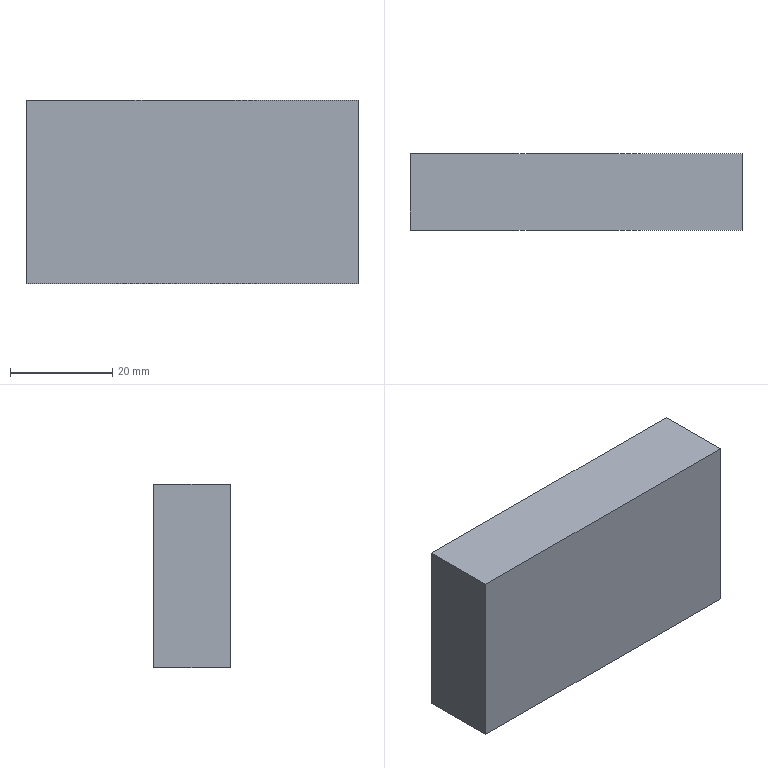Part | SolidWorks | features FlatPattern 1, SMBaseFlange 1, SheetMetal 1 | 1 solid | 6 faces | box 65 x 15 x 36 mm | volume 35100 mm3 | plane 6
STEP:
#1=CARTESIAN_POINT('',(0.,0.,0.));
#2=VERTEX_POINT('',#1);
#3=CARTESIAN_POINT('',(0.,0.,36.));
#4=VERTEX_POINT('',#3);
#5=CARTESIAN_POINT('',(0.,0.,0.));
#6=DIRECTION('',(0.,0.,1.));
#7=VECTOR('',#6,1000.);
#8=LINE('',#5,#7);
#9=EDGE_CURVE('',#2,#4,#8,.T.);
#10=ORIENTED_EDGE('',*,*,#9,.F.);
#11=CARTESIAN_POINT('',(0.,-15.,0.));
#12=VERTEX_POINT('',#11);
#13=CARTESIAN_POINT('',(0.,-15.,0.));
#14=DIRECTION('',(0.,1.,0.));
#15=VECTOR('',#14,1000.);
#16=LINE('',#13,#15);
#17=EDGE_CURVE('',#12,#2,#16,.T.);
#18=ORIENTED_EDGE('',*,*,#17,.F.);
#19=CARTESIAN_POINT('',(0.,-15.,36.));
#20=VERTEX_POINT('',#19);
#21=CARTESIAN_POINT('',(0.,-15.,0.));
#22=DIRECTION('',(0.,0.,1.));
#23=VECTOR('',#22,1000.);
#24=LINE('',#21,#23);
#25=EDGE_CURVE('',#12,#20,#24,.T.);
#26=ORIENTED_EDGE('',*,*,#25,.T.);
#27=CARTESIAN_POINT('',(0.,-15.,36.));
#28=DIRECTION('',(0.,1.,0.));
#29=VECTOR('',#28,1000.);
#30=LINE('',#27,#29);
#31=EDGE_CURVE('',#20,#4,#30,.T.);
#32=ORIENTED_EDGE('',*,*,#31,.T.);
#33=EDGE_LOOP('',(#10,#18,#26,#32));
#34=FACE_OUTER_BOUND('',#33,.T.);
#35=CARTESIAN_POINT('',(0.,-15.,0.));
#36=DIRECTION('',(-1.,0.,0.));
#37=DIRECTION('',(0.,0.,1.));
#38=AXIS2_PLACEMENT_3D('',#35,#36,#37);
#39=PLANE('',#38);
#40=ADVANCED_FACE('',(#34),#39,.T.);
#41=CARTESIAN_POINT('',(65.,0.,0.));
#42=VERTEX_POINT('',#41);
#43=CARTESIAN_POINT('',(0.,0.,0.));
#44=DIRECTION('',(-1.,0.,0.));
#45=VECTOR('',#44,1000.);
#46=LINE('',#43,#45);
#47=EDGE_CURVE('',#42,#2,#46,.T.);
#48=ORIENTED_EDGE('',*,*,#47,.F.);
#49=CARTESIAN_POINT('',(65.,-15.,0.));
#50=VERTEX_POINT('',#49);
#51=CARTESIAN_POINT('',(65.,-15.,0.));
#52=DIRECTION('',(0.,1.,0.));
#53=VECTOR('',#52,1000.);
#54=LINE('',#51,#53);
#55=EDGE_CURVE('',#50,#42,#54,.T.);
#56=ORIENTED_EDGE('',*,*,#55,.F.);
#57=CARTESIAN_POINT('',(0.,-15.,0.));
#58=DIRECTION('',(-1.,0.,0.));
#59=VECTOR('',#58,1000.);
#60=LINE('',#57,#59);
#61=EDGE_CURVE('',#50,#12,#60,.T.);
#62=ORIENTED_EDGE('',*,*,#61,.T.);
#63=ORIENTED_EDGE('',*,*,#17,.T.);
#64=EDGE_LOOP('',(#48,#56,#62,#63));
#65=FACE_OUTER_BOUND('',#64,.T.);
#66=CARTESIAN_POINT('',(0.,-15.,0.));
#67=DIRECTION('',(0.,0.,-1.));
#68=DIRECTION('',(-1.,0.,0.));
#69=AXIS2_PLACEMENT_3D('',#66,#67,#68);
#70=PLANE('',#69);
#71=ADVANCED_FACE('',(#65),#70,.T.);
#72=CARTESIAN_POINT('',(65.,0.,36.));
#73=VERTEX_POINT('',#72);
#74=CARTESIAN_POINT('',(65.,0.,0.));
#75=DIRECTION('',(0.,0.,-1.));
#76=VECTOR('',#75,1000.);
#77=LINE('',#74,#76);
#78=EDGE_CURVE('',#73,#42,#77,.T.);
#79=ORIENTED_EDGE('',*,*,#78,.F.);
#80=CARTESIAN_POINT('',(65.,-15.,36.));
#81=VERTEX_POINT('',#80);
#82=CARTESIAN_POINT('',(65.,-15.,36.));
#83=DIRECTION('',(0.,1.,0.));
#84=VECTOR('',#83,1000.);
#85=LINE('',#82,#84);
#86=EDGE_CURVE('',#81,#73,#85,.T.);
#87=ORIENTED_EDGE('',*,*,#86,.F.);
#88=CARTESIAN_POINT('',(65.,-15.,0.));
#89=DIRECTION('',(0.,0.,-1.));
#90=VECTOR('',#89,1000.);
#91=LINE('',#88,#90);
#92=EDGE_CURVE('',#81,#50,#91,.T.);
#93=ORIENTED_EDGE('',*,*,#92,.T.);
#94=ORIENTED_EDGE('',*,*,#55,.T.);
#95=EDGE_LOOP('',(#79,#87,#93,#94));
#96=FACE_OUTER_BOUND('',#95,.T.);
#97=CARTESIAN_POINT('',(65.,-15.,0.));
#98=DIRECTION('',(1.,0.,0.));
#99=DIRECTION('',(0.,0.,-1.));
#100=AXIS2_PLACEMENT_3D('',#97,#98,#99);
#101=PLANE('',#100);
#102=ADVANCED_FACE('',(#96),#101,.T.);
#103=CARTESIAN_POINT('',(0.,0.,36.));
#104=DIRECTION('',(1.,0.,0.));
#105=VECTOR('',#104,1000.);
#106=LINE('',#103,#105);
#107=EDGE_CURVE('',#4,#73,#106,.T.);
#108=ORIENTED_EDGE('',*,*,#107,.F.);
#109=ORIENTED_EDGE('',*,*,#31,.F.);
#110=CARTESIAN_POINT('',(0.,-15.,36.));
#111=DIRECTION('',(1.,0.,0.));
#112=VECTOR('',#111,1000.);
#113=LINE('',#110,#112);
#114=EDGE_CURVE('',#20,#81,#113,.T.);
#115=ORIENTED_EDGE('',*,*,#114,.T.);
#116=ORIENTED_EDGE('',*,*,#86,.T.);
#117=EDGE_LOOP('',(#108,#109,#115,#116));
#118=FACE_OUTER_BOUND('',#117,.T.);
#119=CARTESIAN_POINT('',(0.,-15.,36.));
#120=DIRECTION('',(0.,0.,1.));
#121=DIRECTION('',(1.,0.,0.));
#122=AXIS2_PLACEMENT_3D('',#119,#120,#121);
#123=PLANE('',#122);
#124=ADVANCED_FACE('',(#118),#123,.T.);
#125=ORIENTED_EDGE('',*,*,#25,.F.);
#126=ORIENTED_EDGE('',*,*,#61,.F.);
#127=ORIENTED_EDGE('',*,*,#92,.F.);
#128=ORIENTED_EDGE('',*,*,#114,.F.);
#129=EDGE_LOOP('',(#125,#126,#127,#128));
#130=FACE_OUTER_BOUND('',#129,.T.);
#131=CARTESIAN_POINT('',(0.,-15.,0.));
#132=DIRECTION('',(0.,1.,0.));
#133=DIRECTION('',(0.,0.,1.));
#134=AXIS2_PLACEMENT_3D('',#131,#132,#133);
#135=PLANE('',#134);
#136=ADVANCED_FACE('',(#130),#135,.F.);
#137=ORIENTED_EDGE('',*,*,#9,.T.);
#138=ORIENTED_EDGE('',*,*,#107,.T.);
#139=ORIENTED_EDGE('',*,*,#78,.T.);
#140=ORIENTED_EDGE('',*,*,#47,.T.);
#141=EDGE_LOOP('',(#137,#138,#139,#140));
#142=FACE_OUTER_BOUND('',#141,.T.);
#143=CARTESIAN_POINT('',(0.,0.,0.));
#144=DIRECTION('',(0.,1.,0.));
#145=DIRECTION('',(0.,0.,1.));
#146=AXIS2_PLACEMENT_3D('',#143,#144,#145);
#147=PLANE('',#146);
#148=ADVANCED_FACE('',(#142),#147,.T.);
#149=CLOSED_SHELL('',(#40,#71,#102,#124,#136,#148));
#150=MANIFOLD_SOLID_BREP('',#149);
#151=CARTESIAN_POINT('',(0.,0.,0.));
#152=DIRECTION('',(0.,0.,1.));
#153=DIRECTION('',(1.,0.,0.));
#154=AXIS2_PLACEMENT_3D('',#151,#152,#153);
#155=(LENGTH_UNIT()NAMED_UNIT(*)SI_UNIT(.MILLI.,.METRE.));
#156=UNCERTAINTY_MEASURE_WITH_UNIT(LENGTH_MEASURE(0.00001),#155,'','');
#157=(NAMED_UNIT(*)PLANE_ANGLE_UNIT()SI_UNIT($,.RADIAN.));
#158=(NAMED_UNIT(*)SI_UNIT($,.STERADIAN.)SOLID_ANGLE_UNIT());
#159=(GEOMETRIC_REPRESENTATION_CONTEXT(3)GLOBAL_UNCERTAINTY_ASSIGNED_CONTEXT((#156))GLOBAL_UNIT_ASSIGNED_CONTEXT((#155,#157,#158))REPRESENTATION_CONTEXT('',''));
#160=ADVANCED_BREP_SHAPE_REPRESENTATION('',(#150,#154),#159);